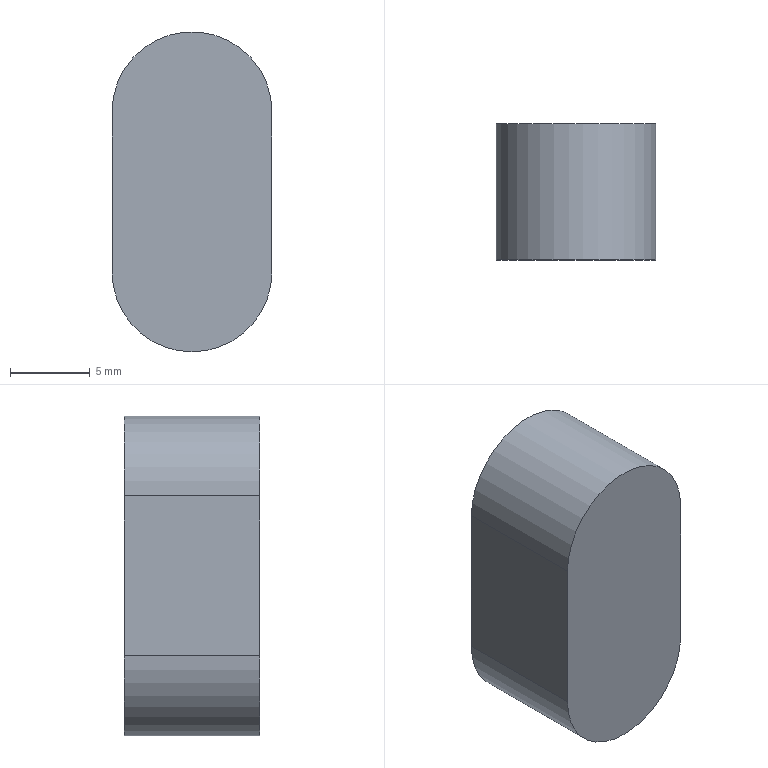Part | SolidWorks | features Extrusion 1 | 1 solid | 7 faces | box 10 x 8.5 x 20 mm | volume 1518 mm3 | plane 4 | cylinder 3 | commonest cylinder face diameters 10 x3
STEP:
#1=CARTESIAN_POINT('',(0.,8.5,-10.));
#2=VERTEX_POINT('',#1);
#3=CARTESIAN_POINT('',(-5.,8.5,-5.));
#4=VERTEX_POINT('',#3);
#5=CARTESIAN_POINT('',(0.,8.5,-5.));
#6=DIRECTION('',(0.,1.,0.));
#7=DIRECTION('',(0.,0.,1.));
#8=AXIS2_PLACEMENT_3D('',#5,#6,#7);
#9=CIRCLE('',#8,5.);
#10=EDGE_CURVE('',#2,#4,#9,.T.);
#11=ORIENTED_EDGE('',*,*,#10,.F.);
#12=CARTESIAN_POINT('',(0.,0.,-10.));
#13=VERTEX_POINT('',#12);
#14=CARTESIAN_POINT('',(0.,8.5,-10.));
#15=DIRECTION('',(0.,-1.,0.));
#16=VECTOR('',#15,1000.);
#17=LINE('',#14,#16);
#18=EDGE_CURVE('',#2,#13,#17,.T.);
#19=ORIENTED_EDGE('',*,*,#18,.T.);
#20=CARTESIAN_POINT('',(-5.,0.,-5.));
#21=VERTEX_POINT('',#20);
#22=CARTESIAN_POINT('',(0.,0.,-5.));
#23=DIRECTION('',(0.,1.,0.));
#24=DIRECTION('',(0.,0.,1.));
#25=AXIS2_PLACEMENT_3D('',#22,#23,#24);
#26=CIRCLE('',#25,5.);
#27=EDGE_CURVE('',#13,#21,#26,.T.);
#28=ORIENTED_EDGE('',*,*,#27,.T.);
#29=CARTESIAN_POINT('',(-5.,8.5,-5.));
#30=DIRECTION('',(0.,-1.,0.));
#31=VECTOR('',#30,1000.);
#32=LINE('',#29,#31);
#33=EDGE_CURVE('',#4,#21,#32,.T.);
#34=ORIENTED_EDGE('',*,*,#33,.F.);
#35=EDGE_LOOP('',(#11,#19,#28,#34));
#36=FACE_OUTER_BOUND('',#35,.T.);
#37=CARTESIAN_POINT('',(0.,8.5,-5.));
#38=DIRECTION('',(0.,-1.,0.));
#39=DIRECTION('',(0.,0.,-1.));
#40=AXIS2_PLACEMENT_3D('',#37,#38,#39);
#41=CYLINDRICAL_SURFACE('',#40,5.);
#42=ADVANCED_FACE('',(#36),#41,.T.);
#43=ORIENTED_EDGE('',*,*,#18,.F.);
#44=CARTESIAN_POINT('',(5.,8.5,-5.));
#45=VERTEX_POINT('',#44);
#46=CARTESIAN_POINT('',(0.,8.5,-5.));
#47=DIRECTION('',(0.,1.,0.));
#48=DIRECTION('',(0.,0.,1.));
#49=AXIS2_PLACEMENT_3D('',#46,#47,#48);
#50=CIRCLE('',#49,5.);
#51=EDGE_CURVE('',#45,#2,#50,.T.);
#52=ORIENTED_EDGE('',*,*,#51,.F.);
#53=CARTESIAN_POINT('',(5.,0.,-5.));
#54=VERTEX_POINT('',#53);
#55=CARTESIAN_POINT('',(5.,8.5,-5.));
#56=DIRECTION('',(0.,-1.,0.));
#57=VECTOR('',#56,1000.);
#58=LINE('',#55,#57);
#59=EDGE_CURVE('',#45,#54,#58,.T.);
#60=ORIENTED_EDGE('',*,*,#59,.T.);
#61=CARTESIAN_POINT('',(0.,0.,-5.));
#62=DIRECTION('',(0.,1.,0.));
#63=DIRECTION('',(0.,0.,1.));
#64=AXIS2_PLACEMENT_3D('',#61,#62,#63);
#65=CIRCLE('',#64,5.);
#66=EDGE_CURVE('',#54,#13,#65,.T.);
#67=ORIENTED_EDGE('',*,*,#66,.T.);
#68=EDGE_LOOP('',(#43,#52,#60,#67));
#69=FACE_OUTER_BOUND('',#68,.T.);
#70=CARTESIAN_POINT('',(0.,8.5,-5.));
#71=DIRECTION('',(0.,-1.,0.));
#72=DIRECTION('',(0.,0.,-1.));
#73=AXIS2_PLACEMENT_3D('',#70,#71,#72);
#74=CYLINDRICAL_SURFACE('',#73,5.);
#75=ADVANCED_FACE('',(#69),#74,.T.);
#76=CARTESIAN_POINT('',(-5.,0.,5.));
#77=VERTEX_POINT('',#76);
#78=CARTESIAN_POINT('',(-5.,0.,-5.));
#79=DIRECTION('',(0.,0.,1.));
#80=VECTOR('',#79,1000.);
#81=LINE('',#78,#80);
#82=EDGE_CURVE('',#21,#77,#81,.T.);
#83=ORIENTED_EDGE('',*,*,#82,.T.);
#84=CARTESIAN_POINT('',(-5.,8.5,5.));
#85=VERTEX_POINT('',#84);
#86=CARTESIAN_POINT('',(-5.,8.5,5.));
#87=DIRECTION('',(0.,-1.,0.));
#88=VECTOR('',#87,1000.);
#89=LINE('',#86,#88);
#90=EDGE_CURVE('',#85,#77,#89,.T.);
#91=ORIENTED_EDGE('',*,*,#90,.F.);
#92=CARTESIAN_POINT('',(-5.,8.5,-5.));
#93=DIRECTION('',(0.,0.,1.));
#94=VECTOR('',#93,1000.);
#95=LINE('',#92,#94);
#96=EDGE_CURVE('',#4,#85,#95,.T.);
#97=ORIENTED_EDGE('',*,*,#96,.F.);
#98=ORIENTED_EDGE('',*,*,#33,.T.);
#99=EDGE_LOOP('',(#83,#91,#97,#98));
#100=FACE_OUTER_BOUND('',#99,.T.);
#101=CARTESIAN_POINT('',(-5.,8.5,-5.));
#102=DIRECTION('',(1.,0.,0.));
#103=DIRECTION('',(0.,0.,-1.));
#104=AXIS2_PLACEMENT_3D('',#101,#102,#103);
#105=PLANE('',#104);
#106=ADVANCED_FACE('',(#100),#105,.F.);
#107=CARTESIAN_POINT('',(5.,0.,5.));
#108=VERTEX_POINT('',#107);
#109=CARTESIAN_POINT('',(0.,0.,5.));
#110=DIRECTION('',(0.,1.,0.));
#111=DIRECTION('',(0.,0.,1.));
#112=AXIS2_PLACEMENT_3D('',#109,#110,#111);
#113=CIRCLE('',#112,5.);
#114=EDGE_CURVE('',#77,#108,#113,.T.);
#115=ORIENTED_EDGE('',*,*,#114,.T.);
#116=CARTESIAN_POINT('',(5.,8.5,5.));
#117=VERTEX_POINT('',#116);
#118=CARTESIAN_POINT('',(5.,8.5,5.));
#119=DIRECTION('',(0.,-1.,0.));
#120=VECTOR('',#119,1000.);
#121=LINE('',#118,#120);
#122=EDGE_CURVE('',#117,#108,#121,.T.);
#123=ORIENTED_EDGE('',*,*,#122,.F.);
#124=CARTESIAN_POINT('',(0.,8.5,5.));
#125=DIRECTION('',(0.,1.,0.));
#126=DIRECTION('',(0.,0.,1.));
#127=AXIS2_PLACEMENT_3D('',#124,#125,#126);
#128=CIRCLE('',#127,5.);
#129=EDGE_CURVE('',#85,#117,#128,.T.);
#130=ORIENTED_EDGE('',*,*,#129,.F.);
#131=ORIENTED_EDGE('',*,*,#90,.T.);
#132=EDGE_LOOP('',(#115,#123,#130,#131));
#133=FACE_OUTER_BOUND('',#132,.T.);
#134=CARTESIAN_POINT('',(0.,8.5,5.));
#135=DIRECTION('',(0.,-1.,0.));
#136=DIRECTION('',(0.,0.,-1.));
#137=AXIS2_PLACEMENT_3D('',#134,#135,#136);
#138=CYLINDRICAL_SURFACE('',#137,5.);
#139=ADVANCED_FACE('',(#133),#138,.T.);
#140=CARTESIAN_POINT('',(5.,0.,5.));
#141=DIRECTION('',(0.,0.,-1.));
#142=VECTOR('',#141,1000.);
#143=LINE('',#140,#142);
#144=EDGE_CURVE('',#108,#54,#143,.T.);
#145=ORIENTED_EDGE('',*,*,#144,.T.);
#146=ORIENTED_EDGE('',*,*,#59,.F.);
#147=CARTESIAN_POINT('',(5.,8.5,5.));
#148=DIRECTION('',(0.,0.,-1.));
#149=VECTOR('',#148,1000.);
#150=LINE('',#147,#149);
#151=EDGE_CURVE('',#117,#45,#150,.T.);
#152=ORIENTED_EDGE('',*,*,#151,.F.);
#153=ORIENTED_EDGE('',*,*,#122,.T.);
#154=EDGE_LOOP('',(#145,#146,#152,#153));
#155=FACE_OUTER_BOUND('',#154,.T.);
#156=CARTESIAN_POINT('',(5.,8.5,5.));
#157=DIRECTION('',(-1.,0.,0.));
#158=DIRECTION('',(0.,0.,1.));
#159=AXIS2_PLACEMENT_3D('',#156,#157,#158);
#160=PLANE('',#159);
#161=ADVANCED_FACE('',(#155),#160,.F.);
#162=ORIENTED_EDGE('',*,*,#51,.T.);
#163=ORIENTED_EDGE('',*,*,#10,.T.);
#164=ORIENTED_EDGE('',*,*,#96,.T.);
#165=ORIENTED_EDGE('',*,*,#129,.T.);
#166=ORIENTED_EDGE('',*,*,#151,.T.);
#167=EDGE_LOOP('',(#162,#163,#164,#165,#166));
#168=FACE_OUTER_BOUND('',#167,.T.);
#169=CARTESIAN_POINT('',(0.,8.5,-5.));
#170=DIRECTION('',(0.,1.,0.));
#171=DIRECTION('',(0.,0.,1.));
#172=AXIS2_PLACEMENT_3D('',#169,#170,#171);
#173=PLANE('',#172);
#174=ADVANCED_FACE('',(#168),#173,.T.);
#175=ORIENTED_EDGE('',*,*,#66,.F.);
#176=ORIENTED_EDGE('',*,*,#144,.F.);
#177=ORIENTED_EDGE('',*,*,#114,.F.);
#178=ORIENTED_EDGE('',*,*,#82,.F.);
#179=ORIENTED_EDGE('',*,*,#27,.F.);
#180=EDGE_LOOP('',(#175,#176,#177,#178,#179));
#181=FACE_OUTER_BOUND('',#180,.T.);
#182=CARTESIAN_POINT('',(0.,0.,-5.));
#183=DIRECTION('',(0.,1.,0.));
#184=DIRECTION('',(0.,0.,1.));
#185=AXIS2_PLACEMENT_3D('',#182,#183,#184);
#186=PLANE('',#185);
#187=ADVANCED_FACE('',(#181),#186,.F.);
#188=CLOSED_SHELL('',(#42,#75,#106,#139,#161,#174,#187));
#189=MANIFOLD_SOLID_BREP('',#188);
#190=CARTESIAN_POINT('',(0.,0.,0.));
#191=DIRECTION('',(0.,0.,1.));
#192=DIRECTION('',(1.,0.,0.));
#193=AXIS2_PLACEMENT_3D('',#190,#191,#192);
#194=(LENGTH_UNIT()NAMED_UNIT(*)SI_UNIT(.MILLI.,.METRE.));
#195=UNCERTAINTY_MEASURE_WITH_UNIT(LENGTH_MEASURE(0.00001),#194,'','');
#196=(NAMED_UNIT(*)PLANE_ANGLE_UNIT()SI_UNIT($,.RADIAN.));
#197=(NAMED_UNIT(*)SI_UNIT($,.STERADIAN.)SOLID_ANGLE_UNIT());
#198=(GEOMETRIC_REPRESENTATION_CONTEXT(3)GLOBAL_UNCERTAINTY_ASSIGNED_CONTEXT((#195))GLOBAL_UNIT_ASSIGNED_CONTEXT((#194,#196,#197))REPRESENTATION_CONTEXT('',''));
#199=ADVANCED_BREP_SHAPE_REPRESENTATION('',(#189,#193),#198);